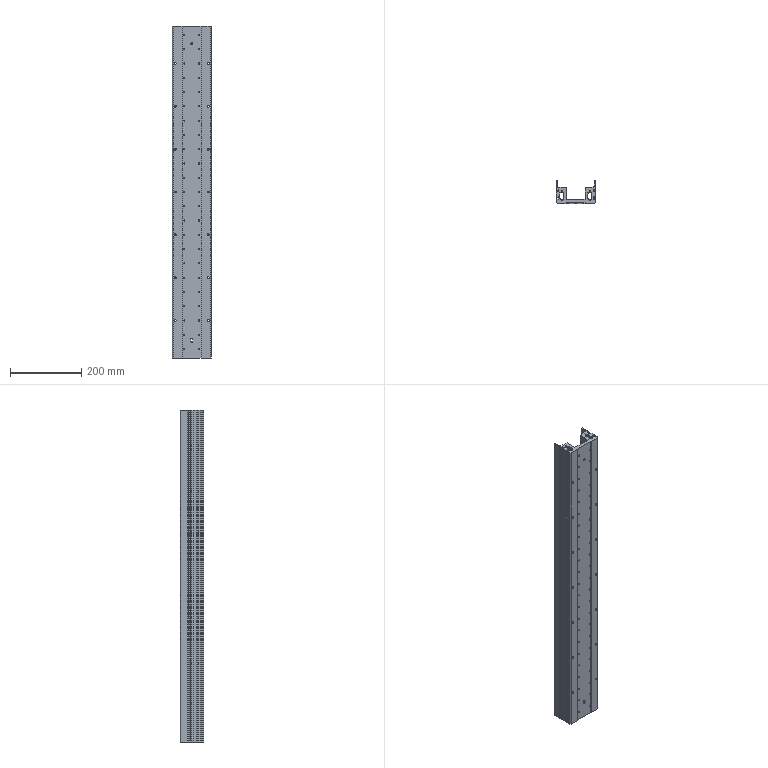Part | SolidWorks | features BaseBody 1 | 1 solid | 558 faces | box 111.5 x 65 x 930 mm | volume 2439001 mm3 | cylinder 299 | plane 195 | cone 64 | commonest cylinder face diameters 3.3 x168 4 x36 5.5 x28 10 x28 6 x21 1 x8